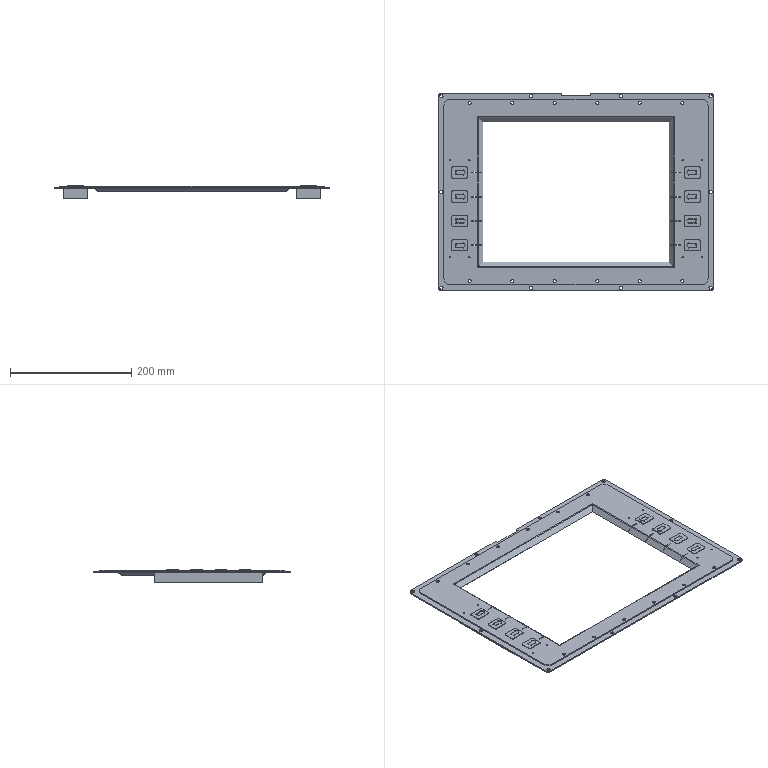Part | SolidWorks | 4 solids | 575 faces | box 455 x 325 x 21.5 mm | volume 462897 mm3 | plane 330 | cylinder 237 | spline 8 | commonest cylinder face diameters 4 x72 5 x69 5.5 x20 2.116 x16 2.5 x16 0.4 x12